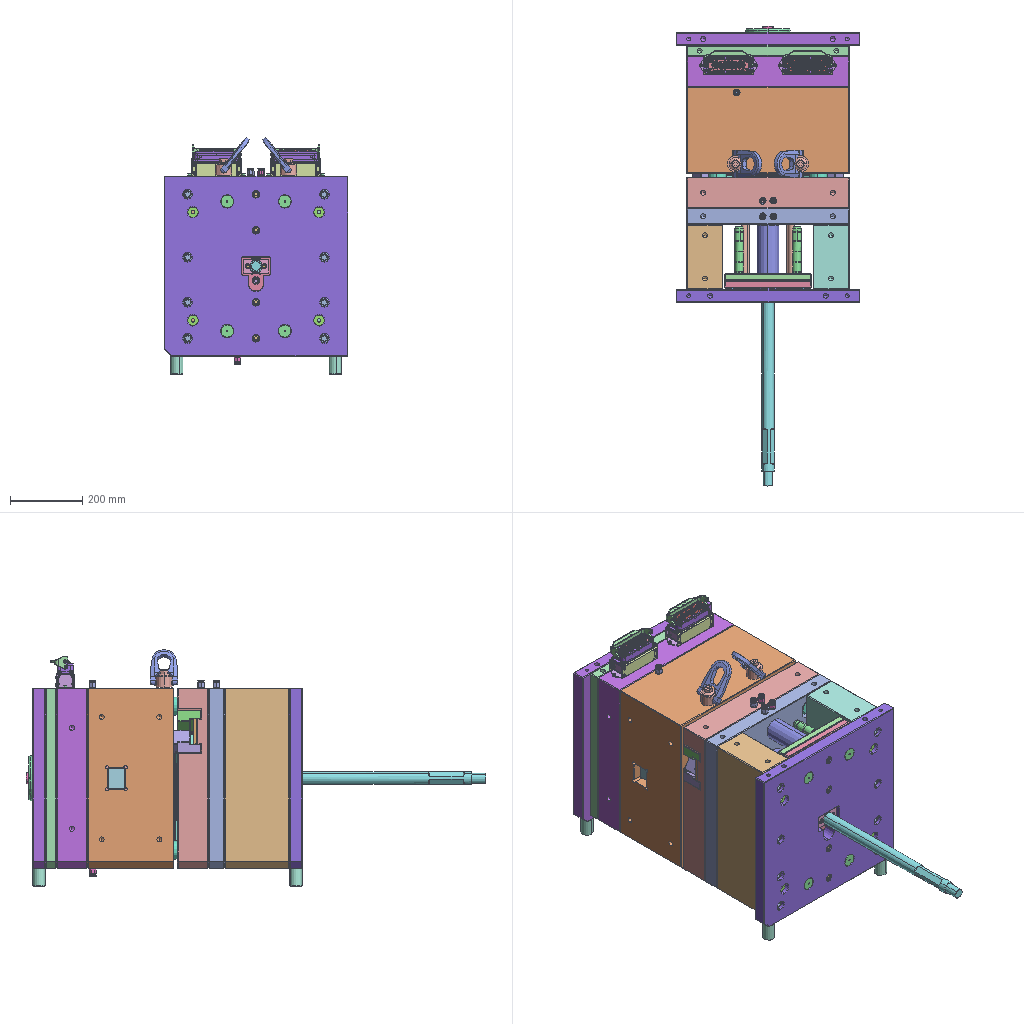Assembly | STEP file | 108 different items | 339 placed | box 510 x 1277 x 657 mm
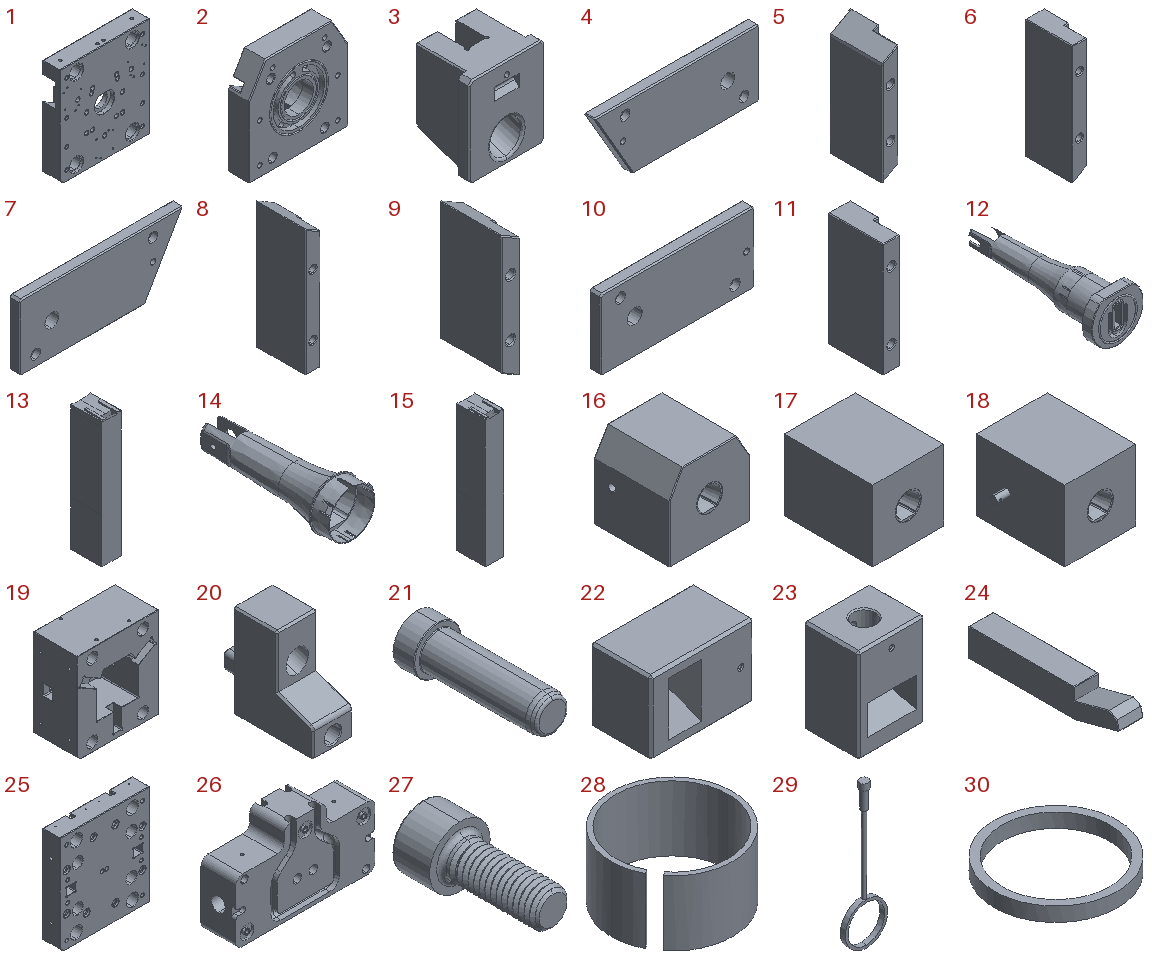Parts list (item | name | quantity | parent item | size | volume):
1 | P2 - 1 cav | x1 | in Montagem do molde TORRE (SUPORTE) VENTILADOR | 450 x 86 x 500 mm | 13008282 mm3
2 | Macho - Torre - 1 cav | x1 | in Montagem do molde TORRE (SUPORTE) VENTILADOR | 230 x 51.25 x 230 mm | 2090171 mm3
3 | Gaveta - Torre - 1 cav | x3 | in Montagem do molde TORRE (SUPORTE) VENTILADOR | 62 x 50 x 73.5 mm | 139216 mm3
4 | Placa de deslize - Torre - 1 - 1 cav | x1 | in Montagem do molde TORRE (SUPORTE) VENTILADOR | 153.211 x 10 x 62 mm | 80124 mm3
5 | Trilho - Torre - 1 cav - 1 | x1 | in Montagem do molde TORRE (SUPORTE) VENTILADOR | 26 x 65 x 141.296 mm | 177227 mm3
6 | Trilho - Torre - 1 cav - 2 | x1 | in Montagem do molde TORRE (SUPORTE) VENTILADOR | 26 x 65 x 164.624 mm | 224436 mm3
7 | Placa de deslize - Torre - 3-  1 cav | x1 | in Montagem do molde TORRE (SUPORTE) VENTILADOR | 153.076 x 10 x 62 mm | 80123 mm3
8 | Trilho - Torre - 1 cav - 3 | x1 | in Montagem do molde TORRE (SUPORTE) VENTILADOR | 26 x 65 x 164.623 mm | 224433 mm3
9 | Trilho - Torre - 1 cav - 4 | x1 | in Montagem do molde TORRE (SUPORTE) VENTILADOR | 26 x 65 x 141.028 mm | 177227 mm3
10 | Placa de deslize - Torre - 4-  1 cav | x1 | in Montagem do molde TORRE (SUPORTE) VENTILADOR | 135 x 10 x 62 mm | 79689 mm3
11 | Trilho - Torre - 1 cav - 5 | x2 | in Montagem do molde TORRE (SUPORTE) VENTILADOR | 26 x 65 x 135 mm | 189332 mm3
12 | Core - Tower - Insert 3 - 1 cav | x1 | in Montagem do molde TORRE (SUPORTE) VENTILADOR | 100 x 274.891 x 90 mm | 522532 mm3
13 | Core - Tower - Drawer insert 1 - 1 cav | x1 | in Montagem do molde TORRE (SUPORTE) VENTILADOR | 16.003 x 25.438 x 104.081 mm | 41692 mm3
14 | Torre - produto - 1 cav | x1 | in Montagem do molde TORRE (SUPORTE) VENTILADOR | 74.278 x 210.114 x 74.851 mm | 69097 mm3
15 | Core - Tower - Drawer insert 2 - 1 cav | x2 | in Montagem do molde TORRE (SUPORTE) VENTILADOR | 16.003 x 25.438 x 113.201 mm | 45404 mm3
16 | Cavidade - Torre - 1 cav | x1 | in Montagem do molde TORRE (SUPORTE) VENTILADOR | 230 x 216.5 x 230 mm | 10150423 mm3
17 | Cavity - Tower - 1 cav - Insert 1 | x1 | in Montagem do molde TORRE (SUPORTE) VENTILADOR | 238 x 250 x 200 mm | 9730114 mm3
18 | Cavity - Tower - 1 cav - Insert 2 | x1 | in Montagem do molde TORRE (SUPORTE) VENTILADOR | 238 x 250 x 200 mm | 9720749 mm3
19 | P1 - 1 cav | x1 | in Montagem do molde TORRE (SUPORTE) VENTILADOR | 450 x 240 x 500 mm | 38190234 mm3
20 | Cunha 2 - Torre - 1 cav | x3 | in Montagem do molde TORRE (SUPORTE) VENTILADOR | 45 x 105 x 105 mm | 266271 mm3
21 | Pino came 1 - Torre - 1 cav | x3 | in Montagem do molde TORRE (SUPORTE) VENTILADOR | 33 x 100 x 33 mm | 52969 mm3
22 | Gaveta - Torre - 4 cav | x1 | in Montagem do molde TORRE (SUPORTE) VENTILADOR | 85 x 50 x 60 mm | 180516 mm3
23 | Gaveta - Torre - 5 cav | x1 | in Montagem do molde TORRE (SUPORTE) VENTILADOR | 60 x 50 x 85 mm | 186270 mm3
24 | Cunha 2 - Torre - 2 cav | x2 | in Montagem do molde TORRE (SUPORTE) VENTILADOR | 40 x 241.767 x 45 mm | 369666 mm3
25 | Manifold - torre - 1 cav | x1 | in Montagem do molde TORRE (SUPORTE) VENTILADOR | 450 x 86 x 500 mm | 13913038 mm3
26 | Manifold-cc | x1 | in Hot runner chamber assembly TOWER | 200 x 50 x 120 mm | 855215 mm3
27 | Parafuso M8 - 20mm | x4 | in Hot runner chamber assembly TOWER | 13 x 28 x 13 mm | 1700 mm3
28 | Jaqueta-A | x1 | in Hot runner chamber assembly TOWER | 37.28 x 37.28 x 20 mm | 3130 mm3
29 | Resist_ncia- reg. - A | x1 | in Hot runner chamber assembly TOWER | 34.4 x 7 x 117.2 mm | 1821 mm3
30 | Resist_ncia-A | x1 | in Hot runner chamber assembly TOWER | 34.4 x 34.4 x 4 mm | 890.436 mm3
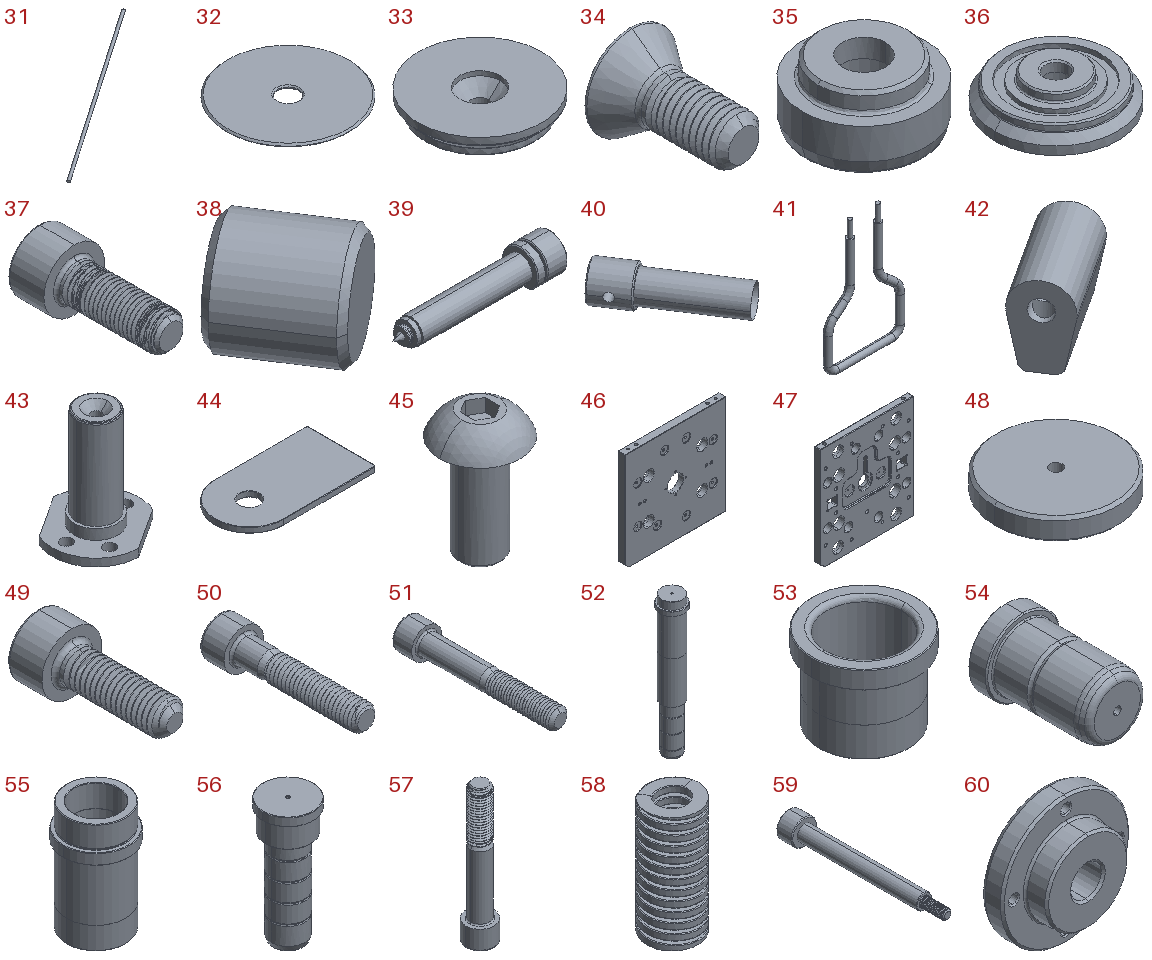31 | Termopar-A | x1 | in Hot runner chamber assembly TOWER | 69.711 x 48.346 x 1 mm | 65.873 mm3
32 | Apoio de Suporte_1-A | x2 | in Hot runner chamber assembly TOWER | 39 x 39 x 1 mm | 1127 mm3
33 | Suporte_1-A | x2 | in Hot runner chamber assembly TOWER | 44 x 44 x 7.51 mm | 9486 mm3
34 | Screw M6 - 10mm flat head | x2 | in Hot runner chamber assembly TOWER | 11.124 x 14 x 11.124 mm | 424.589 mm3
35 | _1971-A | x3 | in Hot runner chamber assembly TOWER | 20 x 20 x 10 mm | 1911 mm3
36 | Suporte Central-A | x3 | in Hot runner chamber assembly TOWER | 44 x 44 x 11 mm | 8128 mm3
37 | Parafuso M6 - 16mm | x3 | in Hot runner chamber assembly TOWER | 10 x 21.9 x 10 mm | 696.612 mm3
38 | Buj_o_1-A | x2 | in Hot runner chamber assembly TOWER | 26.305 x 26.305 x 20 mm | 4786 mm3
39 | BQM F BLOCO VMSMA C1=60mm GATE=1.25mm - TORRE | x2 | in Hot runner chamber assembly TOWER | 96.5 x 22 x 22 mm | 16557 mm3
40 | CPR14030_1-A - longo | x2 | in Hot runner chamber assembly TOWER | - | 9631 mm3
41 | Heater - SUP.INF | x2 | in Hot runner chamber assembly TOWER | 98.5 x 8.5 x 159.25 mm | 21910 mm3
42 | GMBH_3A | x4 | in Hot runner chamber assembly TOWER | 28.047 x 24.519 x 20 mm | 4066 mm3
43 | Corpo da Bucha Acopladora - GRANDE | x1 | in Hot runner chamber assembly TOWER | 68 x 67.975 x 89.05 mm | 70986 mm3
44 | SUPORTE PRENSA CABOS-A | x7 | in Montagem do molde TORRE (SUPORTE) VENTILADOR | 35 x 19 x 1.5 mm | 902.431 mm3
45 | button head socket screw ISO 7380 M5-12-A | x7 | in Montagem do molde TORRE (SUPORTE) VENTILADOR | 9.5 x 9.5 x 14.75 mm | 352.491 mm3
46 | PBS - 1 cav | x1 | in Montagem do molde TORRE (SUPORTE) VENTILADOR | 510 x 36 x 500 mm | 8424078 mm3
47 | Placa fechamento - MANIFOLD - Torre - 1 cav | x1 | in Montagem do molde TORRE (SUPORTE) VENTILADOR | 450 x 30 x 500 mm | 5239142 mm3
48 | SPM 1 | x2 | in Montagem do molde TORRE (SUPORTE) VENTILADOR | 45 x 45 x 8 mm | 12306 mm3
49 | Parafuso M4 - 12mm | x2 | in Montagem do molde TORRE (SUPORTE) VENTILADOR | 7 x 16 x 7 mm | 239.741 mm3
50 | Parafuso M10 - 50mm | x4 | in Montagem do molde TORRE (SUPORTE) VENTILADOR | 16.1 x 60 x 16.1 mm | 4992 mm3
51 | Parafuso M12 - 80mm | x6 | in Montagem do molde TORRE (SUPORTE) VENTILADOR | 18.1 x 91.8 x 18.1 mm | 10767 mm3
52 | Coluna superior CG - CG50196196 | x4 | in Montagem do molde TORRE (SUPORTE) VENTILADOR | 70 x 70 x 395 mm | 1011106 mm3
53 | Bucha B - B50056 | x4 | in Montagem do molde TORRE (SUPORTE) VENTILADOR | 70 x 70 x 55.5 mm | 59351 mm3
54 | Coluna fechamento - torre - 1 cav | x4 | in Montagem do molde TORRE (SUPORTE) VENTILADOR | 60 x 90 x 60 mm | 186134 mm3
55 | Bushing BG - PN_0001 - cut | x4 | in Montagem do molde TORRE (SUPORTE) VENTILADOR | 60 x 60 x 101 mm | 108263 mm3
56 | Upper pillar C- PN_0004 - cut | x4 | in Montagem do molde TORRE (SUPORTE) VENTILADOR | 60 x 60 x 148 mm | 226817 mm3
57 | Parafuso M16 - 100mm - DIN 912 (DIN EM ISO 4762) | x8 | in Montagem do molde TORRE (SUPORTE) VENTILADOR | 24 x 24 x 116.5 mm | 24194 mm3
58 | Mola Vermelha  - R_40-139 - Torre - 1 cav | x8 | in Montagem do molde TORRE (SUPORTE) VENTILADOR | 38 x 38 x 85 mm | 43568 mm3
59 | Parafuso de retorno M12 - Torre - 1 cav | x8 | in Montagem do molde TORRE (SUPORTE) VENTILADOR | 32 x 201 x 32 mm | 61230 mm3
60 | Anel centralizador - Torre 1 cav | x1 | in Montagem do molde TORRE (SUPORTE) VENTILADOR | 124.8 x 41 x 124.8 mm | 308667 mm3
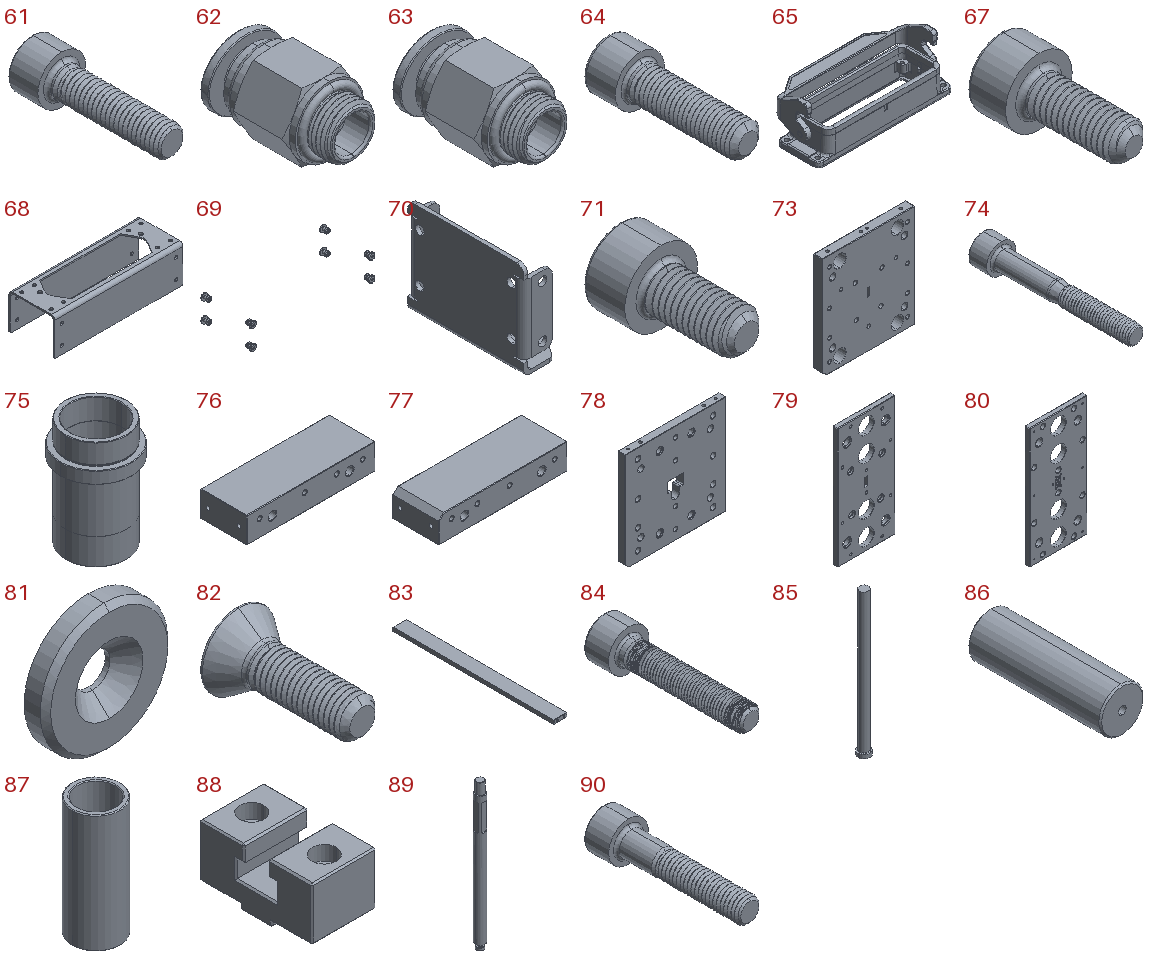61 | Parafuso M8 - 30mm | x4 | in Montagem do molde TORRE (SUPORTE) VENTILADOR | 13 x 38 x 13 mm | 2114 mm3
62 | Quick coupling - 1-4 BSP - COLD | x3 | in Montagem do molde TORRE (SUPORTE) VENTILADOR | 19.63 x 28.5 x 17 mm | 3780 mm3
63 | Quick coupling - 1-4 BSP - HOT | x3 | in Montagem do molde TORRE (SUPORTE) VENTILADOR | 19.63 x 28.5 x 17 mm | 3780 mm3
64 | Parafuso M12 - 40mm | x23 | in Montagem do molde TORRE (SUPORTE) VENTILADOR | 18.1 x 51.8 x 18.1 mm | 6404 mm3
65 | - | x2 | in Female assembly, Montagem macho | 140.01 x 63.21 x 48.7 mm | 56468 mm3
66 | CMM 1224510 - (Inserto miolo f鬥a 24 pinos) | x1 | in Female assembly | - | -
67 | Parafuso M4 - 10mm | x8 | in Female assembly, Montagem macho | 7 x 14 x 7 mm | 220.851 mm3
68 | Corpo | x2 | in Female assembly, Montagem macho | 140 x 50 x 40 mm | 20970 mm3
69 | Rebite cego ISO 15973 - d3.2-6.5. | x2 | in Female assembly, Montagem macho | 131.7 x 52.6 x 27.7 mm | 686.978 mm3
70 | ABA 47-1 - Lateral | x4 | in Female assembly, Montagem macho | 26 x 46.8 x 38.4 mm | 4492 mm3
71 | Parafuso M5 - 10mm | x4 | in Female assembly, Montagem macho | 8.5 x 14.8 x 8.5 mm | 342.133 mm3
72 | CMM 1124510 - (Inserto miolo macho 24 pinos) | x1 | in Montagem macho | - | -
73 | PS - 1 cav | x1 | in Montagem do molde TORRE (SUPORTE) VENTILADOR | 450 x 45 x 500 mm | 9255864 mm3
74 | Parafuso M8 - 60mm | x12 | in Montagem do molde TORRE (SUPORTE) VENTILADOR | 13 x 68 x 13 mm | 3575 mm3
75 | Bushing BG - PN_0002 - cut | x4 | in Montagem do molde TORRE (SUPORTE) VENTILADOR | 70 x 70 x 106.5 mm | 102431 mm3
76 | Spacer block 01 - Tower - 1 cav | x1 | in Montagem do molde TORRE (SUPORTE) VENTILADOR | 500 x 180 x 100 mm | 8680881 mm3
77 | Spacer block 02 - Tower - 1 cav | x1 | in Montagem do molde TORRE (SUPORTE) VENTILADOR | 500 x 180 x 100 mm | 8645281 mm3
78 | PBI - 1 cav | x1 | in Montagem do molde TORRE (SUPORTE) VENTILADOR | 510 x 36 x 500 mm | 8558348 mm3
79 | PE - Torre - 1 cav | x1 | in Montagem do molde TORRE (SUPORTE) VENTILADOR | 240 x 20 x 500 mm | 2018686 mm3
80 | PI - Torre - 1 cav | x1 | in Montagem do molde TORRE (SUPORTE) VENTILADOR | 240 x 20 x 500 mm | 2015685 mm3
81 | Standard stop EP - EP - 2A Polimold - M6 | x6 | in Montagem do molde TORRE (SUPORTE) VENTILADOR | 24 x 4 x 24 mm | 1511 mm3
82 | Screw M6 - 15mm flat head | x6 | in Montagem do molde TORRE (SUPORTE) VENTILADOR | 11.124 x 19 x 11.124 mm | 537.747 mm3
83 | Pino extrator - Torre - 1 cav | x1 | in Montagem do molde TORRE (SUPORTE) VENTILADOR | 35 x 428.85 x 10 mm | 149085 mm3
84 | Parafuso M6 - 30mm | x2 | in Montagem do molde TORRE (SUPORTE) VENTILADOR | 10 x 35.9 x 10 mm | 1008 mm3
85 | Pino extrator A - A_18x315 | x4 | in Montagem do molde TORRE (SUPORTE) VENTILADOR | 24 x 24 x 292 mm | 75901 mm3
86 | Pilar - Torre - 1 cav. | x4 | in Montagem do molde TORRE (SUPORTE) VENTILADOR | 60 x 180 x 60 mm | 505945 mm3
87 | Bucha guia BPR - BPR24074 | x8 | in Montagem do molde TORRE (SUPORTE) VENTILADOR | 30 x 30 x 74 mm | 24346 mm3
88 | BATENTE PLACA EXTRATORA - Torre - 1 cav | x1 | in Montagem do molde TORRE (SUPORTE) VENTILADOR | 40 x 70 x 36 mm | 71533 mm3
89 | Pino extrator para moldes PEQUENOS - SANDRETTO 450T - Torre - 1 cav | x1 | in Montagem do molde TORRE (SUPORTE) VENTILADOR | 35 x 35 x 537.25 mm | 475534 mm3
90 | Parafuso M8 - 40mm | x2 | in Montagem do molde TORRE (SUPORTE) VENTILADOR | 13 x 48 x 13 mm | 2619 mm3
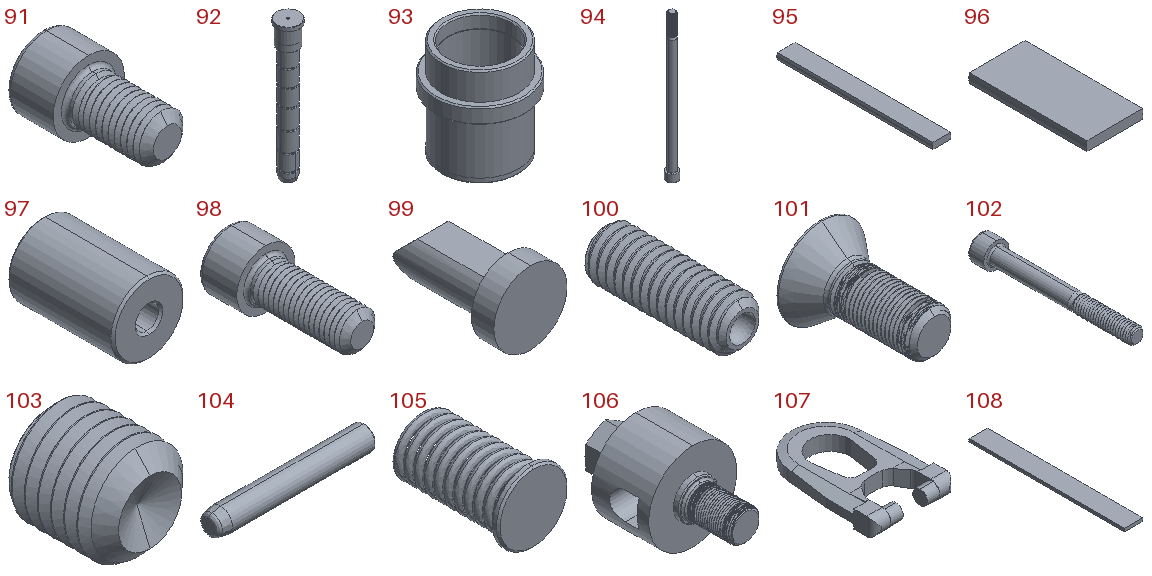91 | Parafuso M12 - 20mm | x10 | in Montagem do molde TORRE (SUPORTE) VENTILADOR | 18.1 x 31.8 x 18.1 mm | 4507 mm3
92 | Coluna inferior | x4 | in Montagem do molde TORRE (SUPORTE) VENTILADOR | 35 x 35 x 211 mm | 105088 mm3
93 | Bucha inferior BEX - BEX2439 | x4 | in Montagem do molde TORRE (SUPORTE) VENTILADOR | 35 x 35 x 38 mm | 10938 mm3
94 | Parafuso M16 - 300mm - DIN 912 (DIN EM ISO 4762) | x8 | in Montagem do molde TORRE (SUPORTE) VENTILADOR | 24 x 24 x 316.5 mm | 64272 mm3
95 | Cooling fin - Tower - 1 cav | x2 | in Montagem do molde TORRE (SUPORTE) VENTILADOR | 6 x 50 x 2 mm | 588.696 mm3
96 | Cooling fin - 2 - Tower - 1 cav | x6 | in Montagem do molde TORRE (SUPORTE) VENTILADOR | 12 x 25 x 2 mm | 597.211 mm3
97 | Mould foot - Tower - 1 cav | x4 | in Montagem do molde TORRE (SUPORTE) VENTILADOR | 34 x 50 x 34 mm | 31705 mm3
98 | Parafuso M12 - 30mm | x4 | in Montagem do molde TORRE (SUPORTE) VENTILADOR | 18.1 x 41.8 x 18.1 mm | 5454 mm3
99 | Trava gavetas - Torre - 1 cav | x3 | in Montagem do molde TORRE (SUPORTE) VENTILADOR | 19.5 x 30.172 x 19.5 mm | 4402 mm3
100 | Plug M6_16 | x3 | in Montagem do molde TORRE (SUPORTE) VENTILADOR | 5.85 x 16 x 5.85 mm | 295.252 mm3
101 | Screw M8 flat head - 20mm | x6 | in Montagem do molde TORRE (SUPORTE) VENTILADOR | 15.374 x 20 x 15.374 mm | 1123 mm3
102 | Parafuso M10 - 90mm | x3 | in Montagem do molde TORRE (SUPORTE) VENTILADOR | 16.1 x 100 x 16.1 mm | 8134 mm3
103 | Plug 3_4'' | x3 | in Montagem do molde TORRE (SUPORTE) VENTILADOR | 19 x 18.901 x 19 mm | 3394 mm3
104 | Pino guia - PNG-0640 - M4 | x2 | in Montagem do molde TORRE (SUPORTE) VENTILADOR | 40 x 6 x 6 mm | 979.582 mm3
105 | Medium blue spring TB - TB16-89 | x3 | in Montagem do molde TORRE (SUPORTE) VENTILADOR | 19 x 30 x 19 mm | 1997 mm3
106 | Parafuso DSR-C - M16 | x2 | in Swivel lifting eye assembly - DSR-C - M16 | 45 x 72 x 45 mm | 55144 mm3
107 | Support bracket - DSR-C | x2 | in Swivel lifting eye assembly - DSR-C - M16 | 76 x 118.25 x 16.8 mm | 64221 mm3
108 | Cooling fin - upper - Tower - 1 cav | x10 | in Montagem do molde TORRE (SUPORTE) VENTILADOR | 12 x 100 x 2 mm | 2389 mm3
Placements (level | parent | child | x y z in mm | rotation matrix by rows), first 202 of 344 lines:
1 | Montagem do molde TORRE (SUPORTE) VENTILADOR | P2 - 1 cav | 183.824 147.313 188.473 | 1 0 0 0 1 0 0 0 1
1 | Montagem do molde TORRE (SUPORTE) VENTILADOR | Macho - Torre - 1 cav | 183.824 238.313 188.473 | 1 0 0 0 1 0 0 0 1
1 | Montagem do molde TORRE (SUPORTE) VENTILADOR | Gaveta - Torre - 1 cav | 12.672 188.313 287.295 | -0.5 0 0.866 0 1 0 -0.866 0 -0.5
1 | Montagem do molde TORRE (SUPORTE) VENTILADOR | Placa de deslize - Torre - 1 - 1 cav | 2.714 178.313 293.047 | 0.866 0 0.5 0 1 0 -0.5 0 0.866
1 | Montagem do molde TORRE (SUPORTE) VENTILADOR | Trilho - Torre - 1 cav - 1 | 147.231 168.313 173.815 | 0.5 0 -0.866 0 1 0 0.866 0 0.5
1 | Montagem do molde TORRE (SUPORTE) VENTILADOR | Trilho - Torre - 1 cav - 2 | -55.398 168.313 362.394 | -0.5 0 0.866 0 1 0 -0.866 0 -0.5
1 | Montagem do molde TORRE (SUPORTE) VENTILADOR | Placa de deslize - Torre - 3-  1 cav | 364.936 178.313 293.045 | 0.866 0 -0.5 0 1 0 0.5 0 0.866
1 | Montagem do molde TORRE (SUPORTE) VENTILADOR | Trilho - Torre - 1 cav - 3 | 275.824 168.313 277.391 | 0.5 0 0.866 0 1 0 -0.866 0 0.5
1 | Montagem do molde TORRE (SUPORTE) VENTILADOR | Trilho - Torre - 1 cav - 4 | 480.226 168.313 323.811 | -0.5 0 -0.866 0 1 0 0.866 0 -0.5
1 | Montagem do molde TORRE (SUPORTE) VENTILADOR | Gaveta - Torre - 1 cav | 354.977 188.313 287.295 | -0.5 0 -0.866 0 1 0 0.866 0 -0.5
1 | Montagem do molde TORRE (SUPORTE) VENTILADOR | Placa de deslize - Torre - 4-  1 cav | 183.824 178.313 5.973 | 0 0 1 0 1 0 -1 0 0
1 | Montagem do molde TORRE (SUPORTE) VENTILADOR | Trilho - Torre - 1 cav - 5 | 152.824 168.313 -61.527 | 1 0 0 0 1 0 0 0 1
1 | Montagem do molde TORRE (SUPORTE) VENTILADOR | Trilho - Torre - 1 cav - 5 | 214.824 168.313 73.473 | -1 0 0 0 1 0 0 0 -1
1 | Montagem do molde TORRE (SUPORTE) VENTILADOR | Gaveta - Torre - 1 cav | 183.824 188.313 -0.0268 | 1 0 0 0 1 0 0 0 1
1 | Montagem do molde TORRE (SUPORTE) VENTILADOR | Core - Tower - Insert 3 - 1 cav | 183.824 238.313 188.473 | 1 0 0 0 1 0 0 0 1
1 | Montagem do molde TORRE (SUPORTE) VENTILADOR | Core - Tower - Drawer insert 1 - 1 cav | 183.824 238.313 188.473 | 1 0 -8e-06 0 1 0 8e-06 0 1
1 | Montagem do molde TORRE (SUPORTE) VENTILADOR | Torre - produto - 1 cav | 183.824 239.643 188.473 | 1 0 0 0 1 0 0 0 1
1 | Montagem do molde TORRE (SUPORTE) VENTILADOR | Core - Tower - Drawer insert 2 - 1 cav | 183.816 238.313 188.485 | -0.5 0 0.866 0 1 0 -0.866 0 -0.5
1 | Montagem do molde TORRE (SUPORTE) VENTILADOR | Core - Tower - Drawer insert 2 - 1 cav | 183.839 238.313 188.475 | -0.5001 0 -0.866 0 1 0 0.866 0 -0.5001
1 | Montagem do molde TORRE (SUPORTE) VENTILADOR | Cavidade - Torre - 1 cav | 183.824 238.313 188.473 | 1 0 0 0 1 0 0 0 1
1 | Montagem do molde TORRE (SUPORTE) VENTILADOR | Cavity - Tower - 1 cav - Insert 1 | 183.824 238.313 188.473 | 1 0 0 0 1 0 0 0 1
1 | Montagem do molde TORRE (SUPORTE) VENTILADOR | Cavity - Tower - 1 cav - Insert 2 | 183.824 238.611 198.358 | 1 0 0 0 0.9982 0.06016 0 -0.06016 0.9982
1 | Montagem do molde TORRE (SUPORTE) VENTILADOR | P1 - 1 cav | 183.824 243.313 188.473 | 1 0 0 0 1 0 0 0 1
1 | Montagem do molde TORRE (SUPORTE) VENTILADOR | Cunha 2 - Torre - 1 cav | 291.324 238.313 250.545 | -0.5 0 -0.866 0 1 0 0.866 0 -0.5
1 | Montagem do molde TORRE (SUPORTE) VENTILADOR | Pino came 1 - Torre - 1 cav | 337.803 193.203 277.38 | 0.9633 -0.2676 -0.02119 0.2676 0.9511 0.1545 -0.02119 -0.1545 0.9878
1 | Montagem do molde TORRE (SUPORTE) VENTILADOR | Cunha 2 - Torre - 1 cav | 76.325 238.313 250.545 | -0.5 0 0.866 0 1 0 -0.866 0 -0.5
1 | Montagem do molde TORRE (SUPORTE) VENTILADOR | Cunha 2 - Torre - 1 cav | 183.824 238.313 73.473 | 1 0 0 0 1 0 0 0 1
1 | Montagem do molde TORRE (SUPORTE) VENTILADOR | Pino came 1 - Torre - 1 cav | 183.824 193.203 19.803 | 0.623 0 0.7822 0.2417 0.9511 -0.1925 -0.744 0.309 0.5925
1 | Montagem do molde TORRE (SUPORTE) VENTILADOR | Pino came 1 - Torre - 1 cav | 29.845 193.203 277.38 | -0.4595 0.2676 0.8469 -0.01496 0.9511 -0.3087 -0.888 -0.1545 -0.433
1 | Montagem do molde TORRE (SUPORTE) VENTILADOR | Gaveta - Torre - 4 cav | 341.324 402.643 188.483 | -1 0 0 0 1 0 0 0 -1
1 | Montagem do molde TORRE (SUPORTE) VENTILADOR | Gaveta - Torre - 5 cav | 26.324 402.643 188.483 | 0 0 1 0 1 0 -1 0 0
1 | Montagem do molde TORRE (SUPORTE) VENTILADOR | Cunha 2 - Torre - 2 cav | 328.824 599.313 188.483 | 0 0 1 0 1 0 -1 0 -0
1 | Montagem do molde TORRE (SUPORTE) VENTILADOR | Cunha 2 - Torre - 2 cav | 38.824 599.313 188.473 | 0 0 -1 0 1 0 1 0 -0
1 | Montagem do molde TORRE (SUPORTE) VENTILADOR | Manifold - torre - 1 cav | 183.824 483.313 188.473 | 1 0 0 0 1 0 0 0 1
1 | Montagem do molde TORRE (SUPORTE) VENTILADOR | Hot runner chamber assembly TOWER | 99.118 441.497 88.706 | 1 0 0 0 1 0 0 0 1
2 | Hot runner chamber assembly TOWER | Manifold-cc | 84.707 103.016 54.768 | 1 0 0 0 1 0 0 0 1
2 | Hot runner chamber assembly TOWER | Parafuso M8 - 20mm | 63.487 114.016 87.518 | 1 0 0 0 1 0 0 0 1
2 | Hot runner chamber assembly TOWER | Parafuso M8 - 20mm | 63.487 114.016 112.018 | 0.9769 0 -0.2136 0 1 0 0.2136 0 0.9769
2 | Hot runner chamber assembly TOWER | Parafuso M8 - 20mm | 105.927 114.016 87.518 | 1 0 0 0 1 0 0 0 1
2 | Hot runner chamber assembly TOWER | Parafuso M8 - 20mm | 105.927 114.016 112.018 | 1 0 0 0 1 0 0 0 1
2 | Hot runner chamber assembly TOWER | Jaqueta-A | 84.707 81.966 99.768 | 0.5446 -0.8387 0 0 0 1 -0.8387 -0.5446 -0
2 | Hot runner chamber assembly TOWER | Resist_ncia- reg. - A | 84.707 144.016 116.768 | 1 0 0 0 1 0 0 0 1
2 | Hot runner chamber assembly TOWER | Resist_ncia-A | 84.707 81.966 99.768 | 0.9859 0.1671 0 0 0 1 0.1671 -0.9859 0
2 | Hot runner chamber assembly TOWER | Termopar-A | 28.079 119.068 103.886 | 0.1736 -0.3217 0.9308 -0.5406 0.7589 0.3632 -0.8232 -0.5662 -0.04215
2 | Hot runner chamber assembly TOWER | Apoio de Suporte_1-A | 71.322 82.016 209.675 | 0.9979 0.06496 0 0 0 1 0.06496 -0.9979 0
2 | Hot runner chamber assembly TOWER | Apoio de Suporte_1-A | 221.321 82.016 209.675 | 0.9979 0.06496 0 0 0 1 0.06496 -0.9979 0
2 | Hot runner chamber assembly TOWER | Suporte_1-A | 97.175 83.016 190.461 | 0.9818 -0.1902 0 0 0 1 -0.1902 -0.9818 0
2 | Hot runner chamber assembly TOWER | Suporte_1-A | 247.175 83.016 190.461 | 0.9818 -0.1902 0 0 0 1 -0.1902 -0.9818 0
2 | Hot runner chamber assembly TOWER | Screw M6 - 10mm flat head | 9.707 120.526 99.768 | 0.9908 0 0.1354 0 1 0 -0.1354 0 0.9908
2 | Hot runner chamber assembly TOWER | Screw M6 - 10mm flat head | 159.707 120.526 99.768 | 0.9908 0 0.1354 0 1 0 -0.1354 0 0.9908
2 | Hot runner chamber assembly TOWER | _1971-A | 84.707 78.016 154.768 | 0.9807 0.1956 0 0 0 1 0.1956 -0.9807 0
2 | Hot runner chamber assembly TOWER | Suporte Central-A | 84.707 78.016 154.768 | 0.905 -0.4255 0 0 0 1 -0.4255 -0.905 -0
2 | Hot runner chamber assembly TOWER | Parafuso M6 - 16mm | 84.707 86.016 154.768 | -0.9794 0 -0.2019 0 -1 0 -0.2019 0 0.9794
2 | Hot runner chamber assembly TOWER | Buj_o_1-A | 163.707 110.503 78.02 | 0.5446 -0.8387 0 0.793 0.515 -0.3255 0.273 0.1773 0.9455
2 | Hot runner chamber assembly TOWER | Buj_o_1-A | 5.707 80.15 97.294 | -0.5446 0.8387 0 -0.09018 -0.05857 0.9942 0.8338 0.5415 0.1075
2 | Hot runner chamber assembly TOWER | BQM F BLOCO VMSMA C1=60mm GATE=1.25mm - TORRE | 96.207 -18.484 99.768 | 0 0 1 1 0 0 0 1 -0
2 | Hot runner chamber assembly TOWER | BQM F BLOCO VMSMA C1=60mm GATE=1.25mm - TORRE | 73.207 -18.484 99.768 | 0 0 -1 1 0 0 0 -1 0
2 | Hot runner chamber assembly TOWER | Suporte Central-A | 0.7066 78.016 69.768 | 0.91 -0.4147 0 0 0 1 -0.4147 -0.91 0
2 | Hot runner chamber assembly TOWER | Suporte Central-A | 168.707 78.016 129.768 | 0.91 -0.4147 0 0 0 1 -0.4147 -0.91 0
2 | Hot runner chamber assembly TOWER | _1971-A | 168.707 78.016 129.768 | 0.9711 0.2386 0 0 0 1 0.2386 -0.9711 0
2 | Hot runner chamber assembly TOWER | _1971-A | 0.7066 78.016 69.768 | 0.9711 0.2386 0 0 0 1 0.2386 -0.9711 0
2 | Hot runner chamber assembly TOWER | Parafuso M6 - 16mm | 0.7066 86.016 69.768 | -0.9794 0 -0.2019 0 -1 0 -0.2019 0 0.9794
2 | Hot runner chamber assembly TOWER | Parafuso M6 - 16mm | 168.707 86.016 129.768 | -0.9794 0 -0.2019 0 -1 0 -0.2019 0 0.9794
2 | Hot runner chamber assembly TOWER | CPR14030_1-A - longo | 193.707 103.016 76.768 | 0.5446 -0.8387 0 0.8387 0.5446 0 0 0 1
2 | Hot runner chamber assembly TOWER | CPR14030_1-A - longo | -24.293 108.235 122.168 | -0.5446 0.8387 0 0.8168 0.5304 -0.2269 -0.1903 -0.1236 -0.9739
2 | Hot runner chamber assembly TOWER | Heater - SUP.INF | 67.207 121.266 199.768 | 1 0 0 0 1 0 0 0 1
2 | Hot runner chamber assembly TOWER | Heater - SUP.INF | 67.207 84.766 199.768 | 1 0 0 0 1 0 0 0 1
2 | Hot runner chamber assembly TOWER | GMBH_3A | 49.707 160.516 109.243 | -0.5446 0.8387 0 0 0 -1 -0.8387 -0.5446 0
2 | Hot runner chamber assembly TOWER | GMBH_3A | 84.707 160.516 109.243 | -0.5446 0.8387 0 0 0 -1 -0.8387 -0.5446 0
2 | Hot runner chamber assembly TOWER | GMBH_3A | 49.707 124.016 109.243 | -0.5446 0.8387 0 0 0 -1 -0.8387 -0.5446 0
2 | Hot runner chamber assembly TOWER | GMBH_3A | 84.707 124.016 109.243 | -0.5446 0.8387 0 0 0 -1 -0.8387 -0.5446 0
2 | Hot runner chamber assembly TOWER | Corpo da Bucha Acopladora - GRANDE | 84.707 81.966 99.768 | 0.8387 0.5446 0 0 0 1 0.5446 -0.8387 -0
1 | Montagem do molde TORRE (SUPORTE) VENTILADOR | SUPORTE PRENSA CABOS-A | 167.824 563.313 353.473 | 1 0 0 0 0 -1 0 1 -0
1 | Montagem do molde TORRE (SUPORTE) VENTILADOR | SUPORTE PRENSA CABOS-A | 133.824 563.313 392.473 | 0 -1 0 0 0 -1 1 0 -0
1 | Montagem do molde TORRE (SUPORTE) VENTILADOR | SUPORTE PRENSA CABOS-A | 127.835 505.513 238.825 | 0.879 0.4769 0 0 0 -1 -0.4769 0.879 0
1 | Montagem do molde TORRE (SUPORTE) VENTILADOR | SUPORTE PRENSA CABOS-A | 121.389 505.513 190.062 | 0.8593 -0.5114 0 0 0 -1 0.5114 0.8593 0
1 | Montagem do molde TORRE (SUPORTE) VENTILADOR | SUPORTE PRENSA CABOS-A | 239.814 505.513 238.825 | -0.879 0.4769 0 0 0 -1 -0.4769 -0.879 0
1 | Montagem do molde TORRE (SUPORTE) VENTILADOR | SUPORTE PRENSA CABOS-A | 246.26 505.513 190.062 | -0.8593 -0.5114 0 0 0 -1 0.5114 -0.8593 -0
1 | Montagem do molde TORRE (SUPORTE) VENTILADOR | button head socket screw ISO 7380 M5-12-A | 127.835 507.013 238.825 | 0.9965 0.08349 0 0 0 1 0.08349 -0.9965 0
1 | Montagem do molde TORRE (SUPORTE) VENTILADOR | button head socket screw ISO 7380 M5-12-A | 121.389 507.013 190.062 | 0.9965 0.08349 0 0 0 1 0.08349 -0.9965 0
1 | Montagem do molde TORRE (SUPORTE) VENTILADOR | button head socket screw ISO 7380 M5-12-A | 246.26 507.013 190.062 | 0.9965 0.08349 0 0 0 1 0.08349 -0.9965 0
1 | Montagem do molde TORRE (SUPORTE) VENTILADOR | button head socket screw ISO 7380 M5-12-A | 239.814 507.013 238.825 | 0.9965 0.08349 0 0 0 1 0.08349 -0.9965 0
1 | Montagem do molde TORRE (SUPORTE) VENTILADOR | button head socket screw ISO 7380 M5-12-A | 167.824 564.813 353.473 | 0.9965 0.08349 0 0 0 1 0.08349 -0.9965 0
1 | Montagem do molde TORRE (SUPORTE) VENTILADOR | button head socket screw ISO 7380 M5-12-A | 133.824 564.813 392.473 | -0.9057 -0.424 0 0 0 1 -0.424 0.9057 0
1 | Montagem do molde TORRE (SUPORTE) VENTILADOR | PBS - 1 cav | 183.824 599.313 188.473 | 1 0 0 0 1 0 0 0 1
1 | Montagem do molde TORRE (SUPORTE) VENTILADOR | Placa fechamento - MANIFOLD - Torre - 1 cav | 183.824 569.313 188.473 | 1 0 0 0 1 0 0 0 1
1 | Montagem do molde TORRE (SUPORTE) VENTILADOR | SPM 1 | 108.824 578.023 188.473 | 0.08497 -0.9964 0 0 0 1 -0.9964 -0.08497 0
1 | Montagem do molde TORRE (SUPORTE) VENTILADOR | SPM 1 | 258.824 578.023 188.473 | 0.08497 -0.9964 0 0 0 1 -0.9964 -0.08497 0
1 | Montagem do molde TORRE (SUPORTE) VENTILADOR | Parafuso M4 - 12mm | 108.824 594.423 188.473 | 0.8715 0 -0.4904 0 -1 0 -0.4904 0 -0.8715
1 | Montagem do molde TORRE (SUPORTE) VENTILADOR | Parafuso M4 - 12mm | 258.824 594.423 188.473 | 0.8715 0 -0.4904 0 -1 0 -0.4904 0 -0.8715
1 | Montagem do molde TORRE (SUPORTE) VENTILADOR | Parafuso M10 - 50mm | 3.824 570.313 188.473 | 1 0 0 0 1 0 0 0 1
1 | Montagem do molde TORRE (SUPORTE) VENTILADOR | Parafuso M10 - 50mm | 28.824 570.313 188.473 | 1 0 0 0 1 0 0 0 1
1 | Montagem do molde TORRE (SUPORTE) VENTILADOR | Parafuso M10 - 50mm | 338.824 570.313 188.483 | 1 0 0 0 1 0 0 0 1
1 | Montagem do molde TORRE (SUPORTE) VENTILADOR | Parafuso M10 - 50mm | 363.824 570.313 188.483 | 1 0 0 0 1 0 0 0 1
1 | Montagem do molde TORRE (SUPORTE) VENTILADOR | Parafuso M12 - 80mm | 248.824 388.313 258.473 | 1 0 0 0 1 0 0 0 1
1 | Montagem do molde TORRE (SUPORTE) VENTILADOR | Parafuso M12 - 80mm | 183.824 388.313 283.473 | 1 0 0 0 1 0 0 0 1
1 | Montagem do molde TORRE (SUPORTE) VENTILADOR | Parafuso M12 - 80mm | 118.824 388.313 258.473 | 1 0 0 0 1 0 0 0 1
1 | Montagem do molde TORRE (SUPORTE) VENTILADOR | Parafuso M12 - 80mm | 98.824 388.313 118.473 | 1 0 0 0 1 0 0 0 1
1 | Montagem do molde TORRE (SUPORTE) VENTILADOR | Parafuso M12 - 80mm | 183.824 388.313 93.473 | 1 0 0 0 1 0 0 0 1
1 | Montagem do molde TORRE (SUPORTE) VENTILADOR | Parafuso M12 - 80mm | 268.824 388.313 118.473 | 1 0 0 0 1 0 0 0 1
1 | Montagem do molde TORRE (SUPORTE) VENTILADOR | Coluna superior CG - CG50196196 | 323.824 92.313 -11.527 | 0.07827 -0.9969 0 0 0 1 -0.9969 -0.07827 0
1 | Montagem do molde TORRE (SUPORTE) VENTILADOR | Coluna superior CG - CG50196196 | 323.824 92.313 388.473 | 0.07827 -0.9969 0 0 0 1 -0.9969 -0.07827 0
1 | Montagem do molde TORRE (SUPORTE) VENTILADOR | Coluna superior CG - CG50196196 | 43.824 92.313 388.473 | 0.07827 -0.9969 0 0 0 1 -0.9969 -0.07827 0
1 | Montagem do molde TORRE (SUPORTE) VENTILADOR | Coluna superior CG - CG50196196 | 43.824 92.313 -11.527 | 0.07827 -0.9969 0 0 0 1 -0.9969 -0.07827 0
1 | Montagem do molde TORRE (SUPORTE) VENTILADOR | Bucha B - B50056 | 323.824 513.813 388.473 | 0.6208 -0.7839 0 0 0 1 -0.7839 -0.6208 -0
1 | Montagem do molde TORRE (SUPORTE) VENTILADOR | Bucha B - B50056 | 43.824 513.813 388.473 | 0.6208 -0.7839 0 0 0 1 -0.7839 -0.6208 -0
1 | Montagem do molde TORRE (SUPORTE) VENTILADOR | Bucha B - B50056 | 323.824 513.813 -11.527 | 0.6208 -0.7839 0 0 0 1 -0.7839 -0.6208 -0
1 | Montagem do molde TORRE (SUPORTE) VENTILADOR | Bucha B - B50056 | 43.824 513.813 -11.527 | 0.6208 -0.7839 0 0 0 1 -0.7839 -0.6208 -0
1 | Montagem do molde TORRE (SUPORTE) VENTILADOR | Coluna fechamento - torre - 1 cav | 323.824 599.313 388.473 | 1 0 0 0 1 0 0 0 1
1 | Montagem do molde TORRE (SUPORTE) VENTILADOR | Coluna fechamento - torre - 1 cav | 43.824 599.313 388.473 | 1 0 0 0 1 0 0 0 1
1 | Montagem do molde TORRE (SUPORTE) VENTILADOR | Coluna fechamento - torre - 1 cav | 43.824 599.313 -11.527 | 1 0 0 0 1 0 0 0 1
1 | Montagem do molde TORRE (SUPORTE) VENTILADOR | Coluna fechamento - torre - 1 cav | 323.824 599.313 -11.527 | 1 0 0 0 1 0 0 0 1
1 | Montagem do molde TORRE (SUPORTE) VENTILADOR | Bushing BG - PN_0001 - cut | 48.824 471.813 88.473 | 0.9324 0.3613 0 0 0 1 0.3613 -0.9324 0
1 | Montagem do molde TORRE (SUPORTE) VENTILADOR | Bushing BG - PN_0001 - cut | 318.824 473.813 88.473 | 0.9324 0.3613 0 0 0 1 0.3613 -0.9324 0
1 | Montagem do molde TORRE (SUPORTE) VENTILADOR | Bushing BG - PN_0001 - cut | 318.824 473.813 288.473 | 0.9324 0.3613 0 0 0 1 0.3613 -0.9324 0
1 | Montagem do molde TORRE (SUPORTE) VENTILADOR | Bushing BG - PN_0001 - cut | 48.824 473.813 288.473 | 0.9324 0.3613 0 0 0 1 0.3613 -0.9324 0
1 | Montagem do molde TORRE (SUPORTE) VENTILADOR | Upper pillar C- PN_0004 - cut | 48.824 464.313 88.473 | 0.971 0.2389 0 0 0 1 0.2389 -0.971 -0
1 | Montagem do molde TORRE (SUPORTE) VENTILADOR | Upper pillar C- PN_0004 - cut | 318.824 464.313 88.473 | 0.971 0.2389 0 0 0 1 0.2389 -0.971 -0
1 | Montagem do molde TORRE (SUPORTE) VENTILADOR | Upper pillar C- PN_0004 - cut | 48.824 464.313 288.473 | 0.971 0.2389 0 0 0 1 0.2389 -0.971 -0
1 | Montagem do molde TORRE (SUPORTE) VENTILADOR | Upper pillar C- PN_0004 - cut | 318.824 464.313 288.473 | -0.9774 -0.2113 0 0 0 1 -0.2113 0.9774 -0
1 | Montagem do molde TORRE (SUPORTE) VENTILADOR | Parafuso M16 - 100mm - DIN 912 (DIN EM ISO 4762) | -6.176 429.313 393.473 | 0.4203 -0.9074 0 0 0 -1 0.9074 0.4203 0
1 | Montagem do molde TORRE (SUPORTE) VENTILADOR | Parafuso M16 - 100mm - DIN 912 (DIN EM ISO 4762) | 373.824 429.313 393.473 | 0.4203 -0.9074 0 0 0 -1 0.9074 0.4203 0
1 | Montagem do molde TORRE (SUPORTE) VENTILADOR | Parafuso M16 - 100mm - DIN 912 (DIN EM ISO 4762) | -1.176 429.313 238.473 | 0.4203 -0.9074 0 0 0 -1 0.9074 0.4203 0
1 | Montagem do molde TORRE (SUPORTE) VENTILADOR | Parafuso M16 - 100mm - DIN 912 (DIN EM ISO 4762) | -1.176 429.313 138.473 | 0.4203 -0.9074 0 0 0 -1 0.9074 0.4203 0
1 | Montagem do molde TORRE (SUPORTE) VENTILADOR | Parafuso M16 - 100mm - DIN 912 (DIN EM ISO 4762) | -6.176 429.313 -21.527 | 0.4203 -0.9074 0 0 0 -1 0.9074 0.4203 0
1 | Montagem do molde TORRE (SUPORTE) VENTILADOR | Parafuso M16 - 100mm - DIN 912 (DIN EM ISO 4762) | 373.824 429.313 -16.527 | 0.4203 -0.9074 0 0 0 -1 0.9074 0.4203 0
1 | Montagem do molde TORRE (SUPORTE) VENTILADOR | Parafuso M16 - 100mm - DIN 912 (DIN EM ISO 4762) | 368.824 429.313 238.473 | 0.4203 -0.9074 0 0 0 -1 0.9074 0.4203 0
1 | Montagem do molde TORRE (SUPORTE) VENTILADOR | Parafuso M16 - 100mm - DIN 912 (DIN EM ISO 4762) | 368.824 429.313 138.473 | 0.4203 -0.9074 0 0 0 -1 0.9074 0.4203 0
1 | Montagem do molde TORRE (SUPORTE) VENTILADOR | Mola Vermelha  - R_40-139 - Torre - 1 cav | 128.753 604.313 358.272 | 0.9997 -0.02632 0 0 0 -1 0.02632 0.9997 -0
1 | Montagem do molde TORRE (SUPORTE) VENTILADOR | Mola Vermelha  - R_40-139 - Torre - 1 cav | 238.9 604.313 358.578 | 0.9997 -0.02632 0 0 0 -1 0.02632 0.9997 -0
1 | Montagem do molde TORRE (SUPORTE) VENTILADOR | Mola Vermelha  - R_40-139 - Torre - 1 cav | -6.151 604.313 283.623 | 0.9997 -0.02632 0 0 0 -1 0.02632 0.9997 -0
1 | Montagem do molde TORRE (SUPORTE) VENTILADOR | Mola Vermelha  - R_40-139 - Torre - 1 cav | 373.678 604.313 283.631 | 0.9997 -0.02632 0 0 0 -1 0.02632 0.9997 -0
1 | Montagem do molde TORRE (SUPORTE) VENTILADOR | Mola Vermelha  - R_40-139 - Torre - 1 cav | -6.254 604.313 93.672 | 0.9997 -0.02632 0 0 0 -1 0.02632 0.9997 -0
1 | Montagem do molde TORRE (SUPORTE) VENTILADOR | Mola Vermelha  - R_40-139 - Torre - 1 cav | 373.829 604.313 93.642 | 0.9997 -0.02632 0 0 0 -1 0.02632 0.9997 -0
1 | Montagem do molde TORRE (SUPORTE) VENTILADOR | Mola Vermelha  - R_40-139 - Torre - 1 cav | 93.811 604.313 48.319 | 0.9997 -0.02632 0 0 0 -1 0.02632 0.9997 -0
1 | Montagem do molde TORRE (SUPORTE) VENTILADOR | Mola Vermelha  - R_40-139 - Torre - 1 cav | 238.721 604.313 18.4 | 0.9997 -0.02632 0 0 0 -1 0.02632 0.9997 -0
1 | Montagem do molde TORRE (SUPORTE) VENTILADOR | Parafuso de retorno M12 - Torre - 1 cav | 238.824 634.313 358.473 | 0.9944 0 0.1056 0 -1 0 0.1056 0 -0.9944
1 | Montagem do molde TORRE (SUPORTE) VENTILADOR | Parafuso de retorno M12 - Torre - 1 cav | 128.824 634.313 358.473 | 0.9944 0 0.1056 0 -1 0 0.1056 0 -0.9944
1 | Montagem do molde TORRE (SUPORTE) VENTILADOR | Parafuso de retorno M12 - Torre - 1 cav | -6.176 634.313 283.473 | 0.9944 0 0.1056 0 -1 0 0.1056 0 -0.9944
1 | Montagem do molde TORRE (SUPORTE) VENTILADOR | Parafuso de retorno M12 - Torre - 1 cav | 373.824 634.313 283.473 | 0.9944 0 0.1056 0 -1 0 0.1056 0 -0.9944
1 | Montagem do molde TORRE (SUPORTE) VENTILADOR | Parafuso de retorno M12 - Torre - 1 cav | -6.176 634.313 93.473 | 0.9944 0 0.1056 0 -1 0 0.1056 0 -0.9944
1 | Montagem do molde TORRE (SUPORTE) VENTILADOR | Parafuso de retorno M12 - Torre - 1 cav | 93.824 634.313 48.473 | 0.9944 0 0.1056 0 -1 0 0.1056 0 -0.9944
1 | Montagem do molde TORRE (SUPORTE) VENTILADOR | Parafuso de retorno M12 - Torre - 1 cav | 238.824 634.313 18.473 | 0.9944 0 0.1056 0 -1 0 0.1056 0 -0.9944
1 | Montagem do molde TORRE (SUPORTE) VENTILADOR | Parafuso de retorno M12 - Torre - 1 cav | 373.824 634.313 93.473 | 0.9944 0 0.1056 0 -1 0 0.1056 0 -0.9944
1 | Montagem do molde TORRE (SUPORTE) VENTILADOR | Anel centralizador - Torre 1 cav | 183.824 604.313 188.473 | 1 0 0 0 1 0 0 0 1
1 | Montagem do molde TORRE (SUPORTE) VENTILADOR | Parafuso M8 - 30mm | 183.824 605.313 137.473 | 1 0 0 0 1 0 0 0 1
1 | Montagem do molde TORRE (SUPORTE) VENTILADOR | Parafuso M8 - 30mm | 132.824 605.313 188.473 | 1 0 0 0 1 0 0 0 1
1 | Montagem do molde TORRE (SUPORTE) VENTILADOR | Parafuso M8 - 30mm | 183.824 605.313 239.473 | 1 0 0 0 1 0 0 0 1
1 | Montagem do molde TORRE (SUPORTE) VENTILADOR | Parafuso M8 - 30mm | 234.824 605.313 188.473 | 1 0 0 0 1 0 0 0 1
1 | Montagem do molde TORRE (SUPORTE) VENTILADOR | Quick coupling - 1-4 BSP - COLD | 96.824 468.313 432.473 | 0.9998 0 -0.01929 -0.01929 0 -0.9998 0 1 0
1 | Montagem do molde TORRE (SUPORTE) VENTILADOR | Quick coupling - 1-4 BSP - HOT | 132.824 468.313 -55.527 | -0.07559 0 -0.9971 0.9971 0 -0.07559 0 -1 -0
1 | Montagem do molde TORRE (SUPORTE) VENTILADOR | Parafuso M12 - 40mm | 108.824 544.313 -11.527 | 1 0 0 0 1 0 0 0 1
1 | Montagem do molde TORRE (SUPORTE) VENTILADOR | Parafuso M12 - 40mm | -16.176 544.313 28.473 | 1 0 0 0 1 0 0 0 1
1 | Montagem do molde TORRE (SUPORTE) VENTILADOR | Parafuso M12 - 40mm | 33.824 544.313 138.473 | 1 0 0 0 1 0 0 0 1
1 | Montagem do molde TORRE (SUPORTE) VENTILADOR | Parafuso M12 - 40mm | 33.824 544.313 238.473 | 1 0 0 0 1 0 0 0 1
1 | Montagem do molde TORRE (SUPORTE) VENTILADOR | Parafuso M12 - 40mm | 183.824 544.313 68.473 | 1 0 0 0 1 0 0 0 1
1 | Montagem do molde TORRE (SUPORTE) VENTILADOR | Parafuso M12 - 40mm | 258.824 544.313 -11.527 | 1 0 0 0 1 0 0 0 1
1 | Montagem do molde TORRE (SUPORTE) VENTILADOR | Parafuso M12 - 40mm | 383.824 544.313 28.473 | 1 0 0 0 1 0 0 0 1
1 | Montagem do molde TORRE (SUPORTE) VENTILADOR | Parafuso M12 - 40mm | 333.824 544.313 138.473 | 1 0 0 0 1 0 0 0 1
1 | Montagem do molde TORRE (SUPORTE) VENTILADOR | Parafuso M12 - 40mm | 333.824 544.313 238.473 | 1 0 0 0 1 0 0 0 1
1 | Montagem do molde TORRE (SUPORTE) VENTILADOR | Parafuso M12 - 40mm | 383.824 544.313 348.473 | 1 0 0 0 1 0 0 0 1
1 | Montagem do molde TORRE (SUPORTE) VENTILADOR | Parafuso M12 - 40mm | 258.824 544.313 388.473 | 1 0 0 0 1 0 0 0 1
1 | Montagem do molde TORRE (SUPORTE) VENTILADOR | Parafuso M12 - 40mm | -16.176 544.313 348.473 | 1 0 0 0 1 0 0 0 1
1 | Montagem do molde TORRE (SUPORTE) VENTILADOR | Parafuso M12 - 40mm | 108.824 544.313 388.473 | 1 0 0 0 1 0 0 0 1
1 | Montagem do molde TORRE (SUPORTE) VENTILADOR | Female assembly | -12.543 477.232 423.532 | 1 0 0 0 1 0 0 0 1
2 | Female assembly | subassembly 2 | 86.867 66.982 72.291 | 1 0 0 0 1 0 0 0 1
2 | Female assembly | CMM 1224510 - (Inserto miolo f鬥a 24 pinos) | 86.867 66.982 72.32 | 1 0 0 0 1 0 0 0 1
2 | Female assembly | Parafuso M4 - 10mm | 151.867 82.982 50.241 | 0.4857 0 -0.8741 -0.8741 0 -0.4857 0 1 0
2 | Female assembly | Parafuso M4 - 10mm | 151.867 50.982 50.241 | 0.4857 0 -0.8741 -0.8741 0 -0.4857 0 1 0
2 | Female assembly | Parafuso M4 - 10mm | 21.867 82.982 50.241 | 0.4857 0 -0.8741 -0.8741 0 -0.4857 0 1 0
2 | Female assembly | Parafuso M4 - 10mm | 21.867 50.982 50.241 | 0.4857 0 -0.8741 -0.8741 0 -0.4857 0 1 0
2 | Female assembly | Corpo | 86.867 66.982 54.941 | 1 0 0 0 1 0 0 0 1
2 | Female assembly | Rebite cego ISO 15973 - d3.2-6.5. | 86.867 66.982 54.941 | 1 0 0 0 1 0 0 0 1
2 | Female assembly | ABA 47-1 - Lateral | 211.867 67.182 54.941 | 1 0 0 0 1 0 0 0 1
2 | Female assembly | ABA 47-1 - Lateral | -38.133 66.982 54.941 | -1 0 0 0 -1 0 0 0 1
2 | Female assembly | Parafuso M5 - 10mm | 162.367 67.082 6.441 | -0.2268 0 -0.9739 -0.9739 0 0.2268 0 1 0
2 | Female assembly | Parafuso M5 - 10mm | 11.367 67.082 6.441 | -0.2268 0 -0.9739 -0.9739 0 0.2268 0 1 0
1 | Montagem do molde TORRE (SUPORTE) VENTILADOR | Montagem macho | 206.457 477.232 423.532 | 1 0 0 0 1 0 0 0 1
2 | Montagem macho | subassembly 2 | 86.867 66.982 72.291 | 1 0 0 0 1 0 0 0 1
2 | Montagem macho | Parafuso M4 - 10mm | 151.867 82.982 50.241 | 0.9245 0 -0.3812 -0.3812 0 -0.9245 0 1 0
2 | Montagem macho | Parafuso M4 - 10mm | 151.867 50.982 50.241 | 0.4857 0 -0.8741 -0.8741 0 -0.4857 0 1 0
2 | Montagem macho | Parafuso M4 - 10mm | 21.867 82.982 50.241 | 0.4857 0 -0.8741 -0.8741 0 -0.4857 0 1 0
2 | Montagem macho | Parafuso M4 - 10mm | 21.867 50.982 50.241 | 0.4857 0 -0.8741 -0.8741 0 -0.4857 0 1 0
2 | Montagem macho | Corpo | 86.867 66.982 54.941 | 1 0 0 0 1 0 0 0 1
2 | Montagem macho | Rebite cego ISO 15973 - d3.2-6.5. | 86.867 66.982 54.941 | 1 0 0 0 1 0 0 0 1
2 | Montagem macho | ABA 47-1 - Lateral | 211.867 67.182 54.941 | 1 0 0 0 1 0 0 0 1
2 | Montagem macho | ABA 47-1 - Lateral | -38.133 66.982 54.941 | -1 0 0 0 -1 0 0 0 1
2 | Montagem macho | Parafuso M5 - 10mm | 162.367 67.082 6.441 | -0.2268 0 -0.9739 -0.9739 0 0.2268 0 1 0
2 | Montagem macho | Parafuso M5 - 10mm | 11.367 67.082 6.441 | -0.2268 0 -0.9739 -0.9739 0 0.2268 0 1 0
2 | Montagem macho | CMM 1124510 - (Inserto miolo macho 24 pinos) | 86.867 66.982 72.286 | 1 0 0 0 1 0 0 0 1
1 | Montagem do molde TORRE (SUPORTE) VENTILADOR | SUPORTE PRENSA CABOS-A | 233.824 563.313 392.473 | 0 -1 0 0 0 -1 1 0 -0
1 | Montagem do molde TORRE (SUPORTE) VENTILADOR | button head socket screw ISO 7380 M5-12-A | 233.824 564.813 392.473 | -0.9057 -0.424 0 0 0 1 -0.424 0.9057 0
1 | Montagem do molde TORRE (SUPORTE) VENTILADOR | PS - 1 cav | 183.824 102.313 188.473 | 1 0 0 0 1 0 0 0 1
1 | Montagem do molde TORRE (SUPORTE) VENTILADOR | Parafuso M12 - 40mm | 123.824 212.313 278.473 | 0.8372 0 0.5469 0 -1 0 0.5469 0 -0.8372
1 | Montagem do molde TORRE (SUPORTE) VENTILADOR | Parafuso M12 - 40mm | 243.824 212.313 278.473 | 0.8372 0 0.5469 0 -1 0 0.5469 0 -0.8372
1 | Montagem do molde TORRE (SUPORTE) VENTILADOR | Parafuso M12 - 40mm | 93.824 212.313 188.473 | 0.8372 0 0.5469 0 -1 0 0.5469 0 -0.8372
1 | Montagem do molde TORRE (SUPORTE) VENTILADOR | Parafuso M12 - 40mm | 273.824 212.313 188.473 | 0.8372 0 0.5469 0 -1 0 0.5469 0 -0.8372
1 | Montagem do molde TORRE (SUPORTE) VENTILADOR | Parafuso M12 - 40mm | 93.824 212.313 98.473 | 0.8372 0 0.5469 0 -1 0 0.5469 0 -0.8372
1 | Montagem do molde TORRE (SUPORTE) VENTILADOR | Parafuso M12 - 40mm | 273.824 212.313 98.473 | 0.8372 0 0.5469 0 -1 0 0.5469 0 -0.8372
1 | Montagem do molde TORRE (SUPORTE) VENTILADOR | Parafuso M8 - 60mm | 224.824 148.313 45.973 | 1 0 0 0 1 0 0 0 1
1 | Montagem do molde TORRE (SUPORTE) VENTILADOR | Parafuso M8 - 60mm | 224.824 148.313 -34.027 | 1 0 0 0 1 0 0 0 1
1 | Montagem do molde TORRE (SUPORTE) VENTILADOR | Parafuso M8 - 60mm | 142.824 148.313 -34.027 | 1 0 0 0 1 0 0 0 1